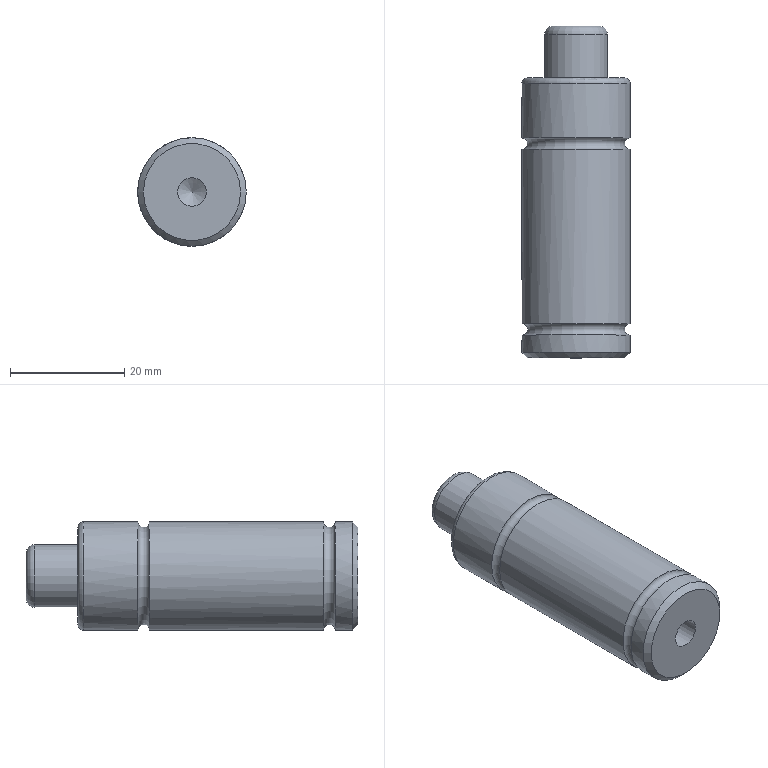Part | STEP file | 1_id822_x_t | 1 solid | 14 faces | box 19 x 58.09 x 19 mm | volume 14020 mm3 | cylinder 5 | torus 4 | plane 3 | cone 2 | commonest cylinder face diameters 19 x3 5 x1 11 x1
STEP:
#1=CARTESIAN_POINT('',(0.,0.,0.));
#2=DIRECTION('',(0.,0.,1.));
#3=DIRECTION('',(1.,0.,0.));
#4=AXIS2_PLACEMENT_3D('',#1,#2,#3);
#5=CARTESIAN_POINT('',(752.425,85.86,-84.184));
#6=VERTEX_POINT('',#5);
#7=CARTESIAN_POINT('',(747.425,85.86,-84.184));
#8=VERTEX_POINT('',#7);
#9=CARTESIAN_POINT('',(749.925,85.86,-84.184));
#10=DIRECTION('',(0.,-1.,0.));
#11=DIRECTION('',(-1.,0.,0.));
#12=AXIS2_PLACEMENT_3D('',#9,#10,#11);
#13=CIRCLE('',#12,2.5);
#14=CARTESIAN_POINT('',(749.925,86.563,-84.184));
#15=DIRECTION('',(0.,-1.,0.));
#16=DIRECTION('',(1.,0.,0.));
#17=AXIS2_PLACEMENT_3D('',#14,#15,#16);
#18=CONICAL_SURFACE('',#17,1.283,1.047);
#19=CARTESIAN_POINT('',(-3.142,0.7025));
#20=DIRECTION('',(1.,0.));
#21=VECTOR('',#20,1.);
#22=LINE('',#19,#21);
#23=(GEOMETRIC_REPRESENTATION_CONTEXT(2)PARAMETRIC_REPRESENTATION_CONTEXT()REPRESENTATION_CONTEXT('',''));
#24=DEFINITIONAL_REPRESENTATION('',(#22),#23);
#25=PCURVE('',#18,#24);
#26=CARTESIAN_POINT('',(749.925,80.86,-84.184));
#27=DIRECTION('',(0.,1.,0.));
#28=DIRECTION('',(1.,0.,0.));
#29=AXIS2_PLACEMENT_3D('',#26,#27,#28);
#30=CYLINDRICAL_SURFACE('',#29,2.5);
#31=CARTESIAN_POINT('',(9.425,5.));
#32=DIRECTION('',(-1.,0.));
#33=VECTOR('',#32,1.);
#34=LINE('',#31,#33);
#35=(GEOMETRIC_REPRESENTATION_CONTEXT(2)PARAMETRIC_REPRESENTATION_CONTEXT()REPRESENTATION_CONTEXT('',''));
#36=DEFINITIONAL_REPRESENTATION('',(#34),#35);
#37=PCURVE('',#30,#36);
#38=SURFACE_CURVE('',#13,(#25,#37),.PCURVE_S1.);
#39=EDGE_CURVE('',#6,#8,#38,.T.);
#40=ORIENTED_EDGE('',*,*,#39,.F.);
#41=CARTESIAN_POINT('',(749.925,87.304,-84.184));
#42=VERTEX_POINT('',#41);
#43=CARTESIAN_POINT('',(749.925,87.304,-84.184));
#44=CARTESIAN_POINT('',(752.425,85.86,-84.184));
#45=B_SPLINE_CURVE_WITH_KNOTS('',1,(#43,#44),.UNSPECIFIED.,.F.,.F.,(2,2),(-1.482,1.405),.PIECEWISE_BEZIER_KNOTS.);
#46=CARTESIAN_POINT('',(0.,0.));
#47=DIRECTION('',(0.,1.));
#48=VECTOR('',#47,1.);
#49=LINE('',#46,#48);
#50=(GEOMETRIC_REPRESENTATION_CONTEXT(2)PARAMETRIC_REPRESENTATION_CONTEXT()REPRESENTATION_CONTEXT('',''));
#51=DEFINITIONAL_REPRESENTATION('',(#49),#50);
#52=PCURVE('',#18,#51);
#53=CARTESIAN_POINT('',(6.283,0.));
#54=DIRECTION('',(0.,1.));
#55=VECTOR('',#54,1.);
#56=LINE('',#53,#55);
#57=(GEOMETRIC_REPRESENTATION_CONTEXT(2)PARAMETRIC_REPRESENTATION_CONTEXT()REPRESENTATION_CONTEXT('',''));
#58=DEFINITIONAL_REPRESENTATION('',(#56),#57);
#59=PCURVE('',#18,#58);
#60=SEAM_CURVE('',#45,(#52,#59),.PCURVE_S1.);
#61=EDGE_CURVE('',#42,#6,#60,.T.);
#62=ORIENTED_EDGE('',*,*,#61,.F.);
#63=ORIENTED_EDGE('',*,*,#61,.T.);
#64=CARTESIAN_POINT('',(749.925,85.86,-84.184));
#65=DIRECTION('',(0.,-1.,0.));
#66=DIRECTION('',(-1.,0.,0.));
#67=AXIS2_PLACEMENT_3D('',#64,#65,#66);
#68=CIRCLE('',#67,2.5);
#69=CARTESIAN_POINT('',(3.142,0.7025));
#70=DIRECTION('',(1.,0.));
#71=VECTOR('',#70,1.);
#72=LINE('',#69,#71);
#73=(GEOMETRIC_REPRESENTATION_CONTEXT(2)PARAMETRIC_REPRESENTATION_CONTEXT()REPRESENTATION_CONTEXT('',''));
#74=DEFINITIONAL_REPRESENTATION('',(#72),#73);
#75=PCURVE('',#18,#74);
#76=CARTESIAN_POINT('',(3.142,5.));
#77=DIRECTION('',(-1.,0.));
#78=VECTOR('',#77,1.);
#79=LINE('',#76,#78);
#80=(GEOMETRIC_REPRESENTATION_CONTEXT(2)PARAMETRIC_REPRESENTATION_CONTEXT()REPRESENTATION_CONTEXT('',''));
#81=DEFINITIONAL_REPRESENTATION('',(#79),#80);
#82=PCURVE('',#30,#81);
#83=SURFACE_CURVE('',#68,(#75,#82),.PCURVE_S1.);
#84=EDGE_CURVE('',#8,#6,#83,.T.);
#85=ORIENTED_EDGE('',*,*,#84,.F.);
#86=EDGE_LOOP('',(#40,#62,#63,#85));
#87=FACE_BOUND('',#86,.F.);
#88=ADVANCED_FACE('',(#87),#18,.F.);
#89=ORIENTED_EDGE('',*,*,#39,.T.);
#90=ORIENTED_EDGE('',*,*,#84,.T.);
#91=CARTESIAN_POINT('',(752.425,60.86,-84.184));
#92=VERTEX_POINT('',#91);
#93=CARTESIAN_POINT('',(752.425,60.86,-84.184));
#94=CARTESIAN_POINT('',(752.425,85.86,-84.184));
#95=B_SPLINE_CURVE_WITH_KNOTS('',1,(#93,#94),.UNSPECIFIED.,.F.,.F.,(2,2),(-20.,5.),.PIECEWISE_BEZIER_KNOTS.);
#96=CARTESIAN_POINT('',(0.,0.));
#97=DIRECTION('',(0.,1.));
#98=VECTOR('',#97,1.);
#99=LINE('',#96,#98);
#100=(GEOMETRIC_REPRESENTATION_CONTEXT(2)PARAMETRIC_REPRESENTATION_CONTEXT()REPRESENTATION_CONTEXT('',''));
#101=DEFINITIONAL_REPRESENTATION('',(#99),#100);
#102=PCURVE('',#30,#101);
#103=CARTESIAN_POINT('',(6.283,0.));
#104=DIRECTION('',(0.,1.));
#105=VECTOR('',#104,1.);
#106=LINE('',#103,#105);
#107=(GEOMETRIC_REPRESENTATION_CONTEXT(2)PARAMETRIC_REPRESENTATION_CONTEXT()REPRESENTATION_CONTEXT('',''));
#108=DEFINITIONAL_REPRESENTATION('',(#106),#107);
#109=PCURVE('',#30,#108);
#110=SEAM_CURVE('',#95,(#102,#109),.PCURVE_S1.);
#111=EDGE_CURVE('',#92,#6,#110,.T.);
#112=ORIENTED_EDGE('',*,*,#111,.F.);
#113=CARTESIAN_POINT('',(749.925,60.86,-84.184));
#114=DIRECTION('',(0.,1.,0.));
#115=DIRECTION('',(1.,0.,0.));
#116=AXIS2_PLACEMENT_3D('',#113,#114,#115);
#117=CIRCLE('',#116,2.5);
#118=CARTESIAN_POINT('',(0.,-20.));
#119=DIRECTION('',(1.,0.));
#120=VECTOR('',#119,1.);
#121=LINE('',#118,#120);
#122=(GEOMETRIC_REPRESENTATION_CONTEXT(2)PARAMETRIC_REPRESENTATION_CONTEXT()REPRESENTATION_CONTEXT('',''));
#123=DEFINITIONAL_REPRESENTATION('',(#121),#122);
#124=PCURVE('',#30,#123);
#125=CARTESIAN_POINT('',(749.925,60.86,-92.684));
#126=DIRECTION('',(0.,1.,0.));
#127=DIRECTION('',(1.,0.,0.));
#128=AXIS2_PLACEMENT_3D('',#125,#126,#127);
#129=PLANE('',#128);
#130=CARTESIAN_POINT('',(0.,-8.5));
#131=DIRECTION('',(1.,0.));
#132=AXIS2_PLACEMENT_2D('',#130,#131);
#133=CIRCLE('',#132,2.5);
#134=(GEOMETRIC_REPRESENTATION_CONTEXT(2)PARAMETRIC_REPRESENTATION_CONTEXT()REPRESENTATION_CONTEXT('',''));
#135=DEFINITIONAL_REPRESENTATION('',(#133),#134);
#136=PCURVE('',#129,#135);
#137=SURFACE_CURVE('',#117,(#124,#136),.PCURVE_S1.);
#138=EDGE_CURVE('',#92,#92,#137,.T.);
#139=ORIENTED_EDGE('',*,*,#138,.T.);
#140=ORIENTED_EDGE('',*,*,#111,.T.);
#141=EDGE_LOOP('',(#89,#90,#112,#139,#140));
#142=FACE_BOUND('',#141,.F.);
#143=ADVANCED_FACE('',(#142),#30,.F.);
#144=CARTESIAN_POINT('',(741.425,60.86,-84.184));
#145=VERTEX_POINT('',#144);
#146=CARTESIAN_POINT('',(749.925,60.86,-84.184));
#147=DIRECTION('',(0.,-1.,0.));
#148=DIRECTION('',(-1.,0.,0.));
#149=AXIS2_PLACEMENT_3D('',#146,#147,#148);
#150=CIRCLE('',#149,8.5);
#151=CARTESIAN_POINT('',(-8.5,-8.5));
#152=CARTESIAN_POINT('',(-8.5,6.222));
#153=CARTESIAN_POINT('',(4.25,-1.139));
#154=CARTESIAN_POINT('',(17.,-8.5));
#155=CARTESIAN_POINT('',(4.25,-15.861));
#156=CARTESIAN_POINT('',(-8.5,-23.222));
#157=CARTESIAN_POINT('',(-8.5,-8.5));
#158=(BOUNDED_CURVE()B_SPLINE_CURVE(2,(#151,#152,#153,#154,#155,#156,#157),.UNSPECIFIED.,.T.,.F.)B_SPLINE_CURVE_WITH_KNOTS((1,2,2,2,2,1),(-2.094,0.,2.094,4.189,6.283,8.378),.UNSPECIFIED.)CURVE()GEOMETRIC_REPRESENTATION_ITEM()RATIONAL_B_SPLINE_CURVE((1.,0.5,1.,0.5,1.,0.5,1.))REPRESENTATION_ITEM(''));
#159=(GEOMETRIC_REPRESENTATION_CONTEXT(2)PARAMETRIC_REPRESENTATION_CONTEXT()REPRESENTATION_CONTEXT('',''));
#160=DEFINITIONAL_REPRESENTATION('',(#158),#159);
#161=PCURVE('',#129,#160);
#162=CARTESIAN_POINT('',(749.925,61.36,-84.184));
#163=DIRECTION('',(0.,1.,0.));
#164=DIRECTION('',(-1.,0.,0.));
#165=AXIS2_PLACEMENT_3D('',#162,#163,#164);
#166=CONICAL_SURFACE('',#165,9.,0.7854);
#167=CARTESIAN_POINT('',(6.283,-0.5));
#168=DIRECTION('',(-1.,0.));
#169=VECTOR('',#168,1.);
#170=LINE('',#167,#169);
#171=(GEOMETRIC_REPRESENTATION_CONTEXT(2)PARAMETRIC_REPRESENTATION_CONTEXT()REPRESENTATION_CONTEXT('',''));
#172=DEFINITIONAL_REPRESENTATION('',(#170),#171);
#173=PCURVE('',#166,#172);
#174=SURFACE_CURVE('',#150,(#161,#173),.PCURVE_S1.);
#175=EDGE_CURVE('',#145,#145,#174,.T.);
#176=ORIENTED_EDGE('',*,*,#175,.T.);
#177=EDGE_LOOP('',(#176));
#178=FACE_BOUND('',#177,.T.);
#179=ORIENTED_EDGE('',*,*,#138,.T.);
#180=EDGE_LOOP('',(#179));
#181=FACE_BOUND('',#180,.T.);
#182=ADVANCED_FACE('',(#178,#181),#129,.F.);
#183=CARTESIAN_POINT('',(740.425,61.86,-84.184));
#184=VERTEX_POINT('',#183);
#185=CARTESIAN_POINT('',(759.425,61.86,-84.184));
#186=VERTEX_POINT('',#185);
#187=CARTESIAN_POINT('',(749.925,61.86,-84.184));
#188=DIRECTION('',(0.,-1.,0.));
#189=DIRECTION('',(-1.,0.,0.));
#190=AXIS2_PLACEMENT_3D('',#187,#188,#189);
#191=CIRCLE('',#190,9.5);
#192=CARTESIAN_POINT('',(6.283,0.5));
#193=DIRECTION('',(-1.,0.));
#194=VECTOR('',#193,1.);
#195=LINE('',#192,#194);
#196=(GEOMETRIC_REPRESENTATION_CONTEXT(2)PARAMETRIC_REPRESENTATION_CONTEXT()REPRESENTATION_CONTEXT('',''));
#197=DEFINITIONAL_REPRESENTATION('',(#195),#196);
#198=PCURVE('',#166,#197);
#199=CARTESIAN_POINT('',(749.925,104.86,-84.184));
#200=DIRECTION('',(0.,1.,0.));
#201=DIRECTION('',(1.,0.,0.));
#202=AXIS2_PLACEMENT_3D('',#199,#200,#201);
#203=CYLINDRICAL_SURFACE('',#202,9.5);
#204=CARTESIAN_POINT('',(3.142,-43.));
#205=DIRECTION('',(-1.,0.));
#206=VECTOR('',#205,1.);
#207=LINE('',#204,#206);
#208=(GEOMETRIC_REPRESENTATION_CONTEXT(2)PARAMETRIC_REPRESENTATION_CONTEXT()REPRESENTATION_CONTEXT('',''));
#209=DEFINITIONAL_REPRESENTATION('',(#207),#208);
#210=PCURVE('',#203,#209);
#211=SURFACE_CURVE('',#191,(#198,#210),.PCURVE_S1.);
#212=EDGE_CURVE('',#184,#186,#211,.T.);
#213=ORIENTED_EDGE('',*,*,#212,.T.);
#214=CARTESIAN_POINT('',(749.925,61.86,-84.184));
#215=DIRECTION('',(0.,-1.,0.));
#216=DIRECTION('',(-1.,0.,0.));
#217=AXIS2_PLACEMENT_3D('',#214,#215,#216);
#218=CIRCLE('',#217,9.5);
#219=CARTESIAN_POINT('',(6.283,0.5));
#220=DIRECTION('',(-1.,0.));
#221=VECTOR('',#220,1.);
#222=LINE('',#219,#221);
#223=(GEOMETRIC_REPRESENTATION_CONTEXT(2)PARAMETRIC_REPRESENTATION_CONTEXT()REPRESENTATION_CONTEXT('',''));
#224=DEFINITIONAL_REPRESENTATION('',(#222),#223);
#225=PCURVE('',#166,#224);
#226=CARTESIAN_POINT('',(9.425,-43.));
#227=DIRECTION('',(-1.,0.));
#228=VECTOR('',#227,1.);
#229=LINE('',#226,#228);
#230=(GEOMETRIC_REPRESENTATION_CONTEXT(2)PARAMETRIC_REPRESENTATION_CONTEXT()REPRESENTATION_CONTEXT('',''));
#231=DEFINITIONAL_REPRESENTATION('',(#229),#230);
#232=PCURVE('',#203,#231);
#233=SURFACE_CURVE('',#218,(#225,#232),.PCURVE_S1.);
#234=EDGE_CURVE('',#186,#184,#233,.T.);
#235=ORIENTED_EDGE('',*,*,#234,.T.);
#236=CARTESIAN_POINT('',(741.425,60.86,-84.184));
#237=CARTESIAN_POINT('',(740.425,61.86,-84.184));
#238=B_SPLINE_CURVE_WITH_KNOTS('',1,(#236,#237),.UNSPECIFIED.,.F.,.F.,(2,2),(-0.7071,0.7071),.PIECEWISE_BEZIER_KNOTS.);
#239=CARTESIAN_POINT('',(0.,0.));
#240=DIRECTION('',(0.,1.));
#241=VECTOR('',#240,1.);
#242=LINE('',#239,#241);
#243=(GEOMETRIC_REPRESENTATION_CONTEXT(2)PARAMETRIC_REPRESENTATION_CONTEXT()REPRESENTATION_CONTEXT('',''));
#244=DEFINITIONAL_REPRESENTATION('',(#242),#243);
#245=PCURVE('',#166,#244);
#246=CARTESIAN_POINT('',(6.283,0.));
#247=DIRECTION('',(0.,1.));
#248=VECTOR('',#247,1.);
#249=LINE('',#246,#248);
#250=(GEOMETRIC_REPRESENTATION_CONTEXT(2)PARAMETRIC_REPRESENTATION_CONTEXT()REPRESENTATION_CONTEXT('',''));
#251=DEFINITIONAL_REPRESENTATION('',(#249),#250);
#252=PCURVE('',#166,#251);
#253=SEAM_CURVE('',#238,(#245,#252),.PCURVE_S1.);
#254=EDGE_CURVE('',#145,#184,#253,.T.);
#255=ORIENTED_EDGE('',*,*,#254,.F.);
#256=ORIENTED_EDGE('',*,*,#175,.F.);
#257=ORIENTED_EDGE('',*,*,#254,.T.);
#258=EDGE_LOOP('',(#213,#235,#255,#256,#257));
#259=FACE_BOUND('',#258,.T.);
#260=ADVANCED_FACE('',(#259),#166,.T.);
#261=CARTESIAN_POINT('',(759.425,64.86,-84.184));
#262=VERTEX_POINT('',#261);
#263=CARTESIAN_POINT('',(749.925,64.86,-84.184));
#264=DIRECTION('',(0.,1.,0.));
#265=DIRECTION('',(1.,0.,0.));
#266=AXIS2_PLACEMENT_3D('',#263,#264,#265);
#267=CIRCLE('',#266,9.5);
#268=CARTESIAN_POINT('',(0.,-40.));
#269=DIRECTION('',(1.,0.));
#270=VECTOR('',#269,1.);
#271=LINE('',#268,#270);
#272=(GEOMETRIC_REPRESENTATION_CONTEXT(2)PARAMETRIC_REPRESENTATION_CONTEXT()REPRESENTATION_CONTEXT('',''));
#273=DEFINITIONAL_REPRESENTATION('',(#271),#272);
#274=PCURVE('',#203,#273);
#275=CARTESIAN_POINT('',(749.925,65.86,-84.184));
#276=DIRECTION('',(0.,-1.,0.));
#277=DIRECTION('',(1.,0.,0.));
#278=AXIS2_PLACEMENT_3D('',#275,#276,#277);
#279=TOROIDAL_SURFACE('',#278,9.5,1.);
#280=CARTESIAN_POINT('',(6.283,1.571));
#281=DIRECTION('',(-1.,0.));
#282=VECTOR('',#281,1.);
#283=LINE('',#280,#282);
#284=(GEOMETRIC_REPRESENTATION_CONTEXT(2)PARAMETRIC_REPRESENTATION_CONTEXT()REPRESENTATION_CONTEXT('',''));
#285=DEFINITIONAL_REPRESENTATION('',(#283),#284);
#286=PCURVE('',#279,#285);
#287=SURFACE_CURVE('',#267,(#274,#286),.PCURVE_S1.);
#288=EDGE_CURVE('',#262,#262,#287,.T.);
#289=ORIENTED_EDGE('',*,*,#288,.F.);
#290=CARTESIAN_POINT('',(759.425,61.86,-84.184));
#291=CARTESIAN_POINT('',(759.425,64.86,-84.184));
#292=B_SPLINE_CURVE_WITH_KNOTS('',1,(#290,#291),.UNSPECIFIED.,.F.,.F.,(2,2),(-43.,-40.),.PIECEWISE_BEZIER_KNOTS.);
#293=CARTESIAN_POINT('',(0.,0.));
#294=DIRECTION('',(0.,1.));
#295=VECTOR('',#294,1.);
#296=LINE('',#293,#295);
#297=(GEOMETRIC_REPRESENTATION_CONTEXT(2)PARAMETRIC_REPRESENTATION_CONTEXT()REPRESENTATION_CONTEXT('',''));
#298=DEFINITIONAL_REPRESENTATION('',(#296),#297);
#299=PCURVE('',#203,#298);
#300=CARTESIAN_POINT('',(6.283,0.));
#301=DIRECTION('',(0.,1.));
#302=VECTOR('',#301,1.);
#303=LINE('',#300,#302);
#304=(GEOMETRIC_REPRESENTATION_CONTEXT(2)PARAMETRIC_REPRESENTATION_CONTEXT()REPRESENTATION_CONTEXT('',''));
#305=DEFINITIONAL_REPRESENTATION('',(#303),#304);
#306=PCURVE('',#203,#305);
#307=SEAM_CURVE('',#292,(#299,#306),.PCURVE_S1.);
#308=EDGE_CURVE('',#186,#262,#307,.T.);
#309=ORIENTED_EDGE('',*,*,#308,.F.);
#310=ORIENTED_EDGE('',*,*,#212,.F.);
#311=ORIENTED_EDGE('',*,*,#234,.F.);
#312=ORIENTED_EDGE('',*,*,#308,.T.);
#313=EDGE_LOOP('',(#289,#309,#310,#311,#312));
#314=FACE_BOUND('',#313,.T.);
#315=ADVANCED_FACE('',(#314),#203,.T.);
#316=CARTESIAN_POINT('',(759.425,66.86,-84.184));
#317=VERTEX_POINT('',#316);
#318=CARTESIAN_POINT('',(749.925,66.86,-84.184));
#319=DIRECTION('',(0.,-1.,0.));
#320=DIRECTION('',(1.,0.,0.));
#321=AXIS2_PLACEMENT_3D('',#318,#319,#320);
#322=CIRCLE('',#321,9.5);
#323=CARTESIAN_POINT('',(0.,4.712));
#324=DIRECTION('',(1.,0.));
#325=VECTOR('',#324,1.);
#326=LINE('',#323,#325);
#327=(GEOMETRIC_REPRESENTATION_CONTEXT(2)PARAMETRIC_REPRESENTATION_CONTEXT()REPRESENTATION_CONTEXT('',''));
#328=DEFINITIONAL_REPRESENTATION('',(#326),#327);
#329=PCURVE('',#279,#328);
#330=CARTESIAN_POINT('',(749.925,104.86,-84.184));
#331=DIRECTION('',(0.,1.,0.));
#332=DIRECTION('',(1.,0.,0.));
#333=AXIS2_PLACEMENT_3D('',#330,#331,#332);
#334=CYLINDRICAL_SURFACE('',#333,9.5);
#335=CARTESIAN_POINT('',(6.283,-38.));
#336=DIRECTION('',(-1.,0.));
#337=VECTOR('',#336,1.);
#338=LINE('',#335,#337);
#339=(GEOMETRIC_REPRESENTATION_CONTEXT(2)PARAMETRIC_REPRESENTATION_CONTEXT()REPRESENTATION_CONTEXT('',''));
#340=DEFINITIONAL_REPRESENTATION('',(#338),#339);
#341=PCURVE('',#334,#340);
#342=SURFACE_CURVE('',#322,(#329,#341),.PCURVE_S1.);
#343=EDGE_CURVE('',#317,#317,#342,.T.);
#344=ORIENTED_EDGE('',*,*,#343,.F.);
#345=CARTESIAN_POINT('',(759.425,64.86,-84.184));
#346=CARTESIAN_POINT('',(759.032,64.86,-84.184));
#347=CARTESIAN_POINT('',(758.64,65.036,-84.184));
#348=CARTESIAN_POINT('',(758.339,65.389,-84.184));
#349=CARTESIAN_POINT('',(758.223,65.86,-84.184));
#350=CARTESIAN_POINT('',(758.339,66.332,-84.184));
#351=CARTESIAN_POINT('',(758.64,66.684,-84.184));
#352=CARTESIAN_POINT('',(759.032,66.86,-84.184));
#353=CARTESIAN_POINT('',(759.425,66.86,-84.184));
#354=B_SPLINE_CURVE_WITH_KNOTS('',8,(#345,#346,#347,#348,#349,#350,#351,#352,#353),.UNSPECIFIED.,.F.,.F.,(9,9),(1.571,4.712),.PIECEWISE_BEZIER_KNOTS.);
#355=CARTESIAN_POINT('',(0.,0.));
#356=DIRECTION('',(0.,1.));
#357=VECTOR('',#356,1.);
#358=LINE('',#355,#357);
#359=(GEOMETRIC_REPRESENTATION_CONTEXT(2)PARAMETRIC_REPRESENTATION_CONTEXT()REPRESENTATION_CONTEXT('',''));
#360=DEFINITIONAL_REPRESENTATION('',(#358),#359);
#361=PCURVE('',#279,#360);
#362=CARTESIAN_POINT('',(6.283,0.));
#363=DIRECTION('',(0.,1.));
#364=VECTOR('',#363,1.);
#365=LINE('',#362,#364);
#366=(GEOMETRIC_REPRESENTATION_CONTEXT(2)PARAMETRIC_REPRESENTATION_CONTEXT()REPRESENTATION_CONTEXT('',''));
#367=DEFINITIONAL_REPRESENTATION('',(#365),#366);
#368=PCURVE('',#279,#367);
#369=SEAM_CURVE('',#354,(#361,#368),.PCURVE_S1.);
#370=EDGE_CURVE('',#262,#317,#369,.T.);
#371=ORIENTED_EDGE('',*,*,#370,.F.);
#372=ORIENTED_EDGE('',*,*,#288,.F.);
#373=ORIENTED_EDGE('',*,*,#370,.T.);
#374=EDGE_LOOP('',(#344,#371,#372,#373));
#375=FACE_BOUND('',#374,.F.);
#376=ADVANCED_FACE('',(#375),#279,.F.);
#377=CARTESIAN_POINT('',(759.425,97.36,-84.184));
#378=VERTEX_POINT('',#377);
#379=CARTESIAN_POINT('',(740.425,97.36,-84.184));
#380=VERTEX_POINT('',#379);
#381=CARTESIAN_POINT('',(749.925,97.36,-84.184));
#382=DIRECTION('',(0.,1.,0.));
#383=DIRECTION('',(-1.,0.,0.));
#384=AXIS2_PLACEMENT_3D('',#381,#382,#383);
#385=CIRCLE('',#384,9.5);
#386=CARTESIAN_POINT('',(-3.142,-7.5));
#387=DIRECTION('',(1.,0.));
#388=VECTOR('',#387,1.);
#389=LINE('',#386,#388);
#390=(GEOMETRIC_REPRESENTATION_CONTEXT(2)PARAMETRIC_REPRESENTATION_CONTEXT()REPRESENTATION_CONTEXT('',''));
#391=DEFINITIONAL_REPRESENTATION('',(#389),#390);
#392=PCURVE('',#334,#391);
#393=CARTESIAN_POINT('',(749.925,98.36,-84.184));
#394=DIRECTION('',(0.,-1.,0.));
#395=DIRECTION('',(1.,0.,0.));
#396=AXIS2_PLACEMENT_3D('',#393,#394,#395);
#397=TOROIDAL_SURFACE('',#396,9.5,1.);
#398=CARTESIAN_POINT('',(9.425,1.571));
#399=DIRECTION('',(-1.,0.));
#400=VECTOR('',#399,1.);
#401=LINE('',#398,#400);
#402=(GEOMETRIC_REPRESENTATION_CONTEXT(2)PARAMETRIC_REPRESENTATION_CONTEXT()REPRESENTATION_CONTEXT('',''));
#403=DEFINITIONAL_REPRESENTATION('',(#401),#402);
#404=PCURVE('',#397,#403);
#405=SURFACE_CURVE('',#385,(#392,#404),.PCURVE_S1.);
#406=EDGE_CURVE('',#378,#380,#405,.T.);
#407=ORIENTED_EDGE('',*,*,#406,.F.);
#408=CARTESIAN_POINT('',(759.425,66.86,-84.184));
#409=CARTESIAN_POINT('',(759.425,97.36,-84.184));
#410=B_SPLINE_CURVE_WITH_KNOTS('',1,(#408,#409),.UNSPECIFIED.,.F.,.F.,(2,2),(-38.,-7.5),.PIECEWISE_BEZIER_KNOTS.);
#411=CARTESIAN_POINT('',(0.,0.));
#412=DIRECTION('',(0.,1.));
#413=VECTOR('',#412,1.);
#414=LINE('',#411,#413);
#415=(GEOMETRIC_REPRESENTATION_CONTEXT(2)PARAMETRIC_REPRESENTATION_CONTEXT()REPRESENTATION_CONTEXT('',''));
#416=DEFINITIONAL_REPRESENTATION('',(#414),#415);
#417=PCURVE('',#334,#416);
#418=CARTESIAN_POINT('',(6.283,0.));
#419=DIRECTION('',(0.,1.));
#420=VECTOR('',#419,1.);
#421=LINE('',#418,#420);
#422=(GEOMETRIC_REPRESENTATION_CONTEXT(2)PARAMETRIC_REPRESENTATION_CONTEXT()REPRESENTATION_CONTEXT('',''));
#423=DEFINITIONAL_REPRESENTATION('',(#421),#422);
#424=PCURVE('',#334,#423);
#425=SEAM_CURVE('',#410,(#417,#424),.PCURVE_S1.);
#426=EDGE_CURVE('',#317,#378,#425,.T.);
#427=ORIENTED_EDGE('',*,*,#426,.F.);
#428=ORIENTED_EDGE('',*,*,#343,.F.);
#429=ORIENTED_EDGE('',*,*,#426,.T.);
#430=CARTESIAN_POINT('',(749.925,97.36,-84.184));
#431=DIRECTION('',(0.,1.,0.));
#432=DIRECTION('',(-1.,0.,0.));
#433=AXIS2_PLACEMENT_3D('',#430,#431,#432);
#434=CIRCLE('',#433,9.5);
#435=CARTESIAN_POINT('',(3.142,-7.5));
#436=DIRECTION('',(1.,0.));
#437=VECTOR('',#436,1.);
#438=LINE('',#435,#437);
#439=(GEOMETRIC_REPRESENTATION_CONTEXT(2)PARAMETRIC_REPRESENTATION_CONTEXT()REPRESENTATION_CONTEXT('',''));
#440=DEFINITIONAL_REPRESENTATION('',(#438),#439);
#441=PCURVE('',#334,#440);
#442=CARTESIAN_POINT('',(9.425,1.571));
#443=DIRECTION('',(-1.,0.));
#444=VECTOR('',#443,1.);
#445=LINE('',#442,#444);
#446=(GEOMETRIC_REPRESENTATION_CONTEXT(2)PARAMETRIC_REPRESENTATION_CONTEXT()REPRESENTATION_CONTEXT('',''));
#447=DEFINITIONAL_REPRESENTATION('',(#445),#446);
#448=PCURVE('',#397,#447);
#449=SURFACE_CURVE('',#434,(#441,#448),.PCURVE_S1.);
#450=EDGE_CURVE('',#380,#378,#449,.T.);
#451=ORIENTED_EDGE('',*,*,#450,.F.);
#452=EDGE_LOOP('',(#407,#427,#428,#429,#451));
#453=FACE_BOUND('',#452,.T.);
#454=ADVANCED_FACE('',(#453),#334,.T.);
#455=CARTESIAN_POINT('',(740.425,99.36,-84.184));
#456=VERTEX_POINT('',#455);
#457=CARTESIAN_POINT('',(759.425,99.36,-84.184));
#458=VERTEX_POINT('',#457);
#459=CARTESIAN_POINT('',(749.925,99.36,-84.184));
#460=DIRECTION('',(0.,-1.,0.));
#461=DIRECTION('',(-1.,0.,0.));
#462=AXIS2_PLACEMENT_3D('',#459,#460,#461);
#463=CIRCLE('',#462,9.5);
#464=CARTESIAN_POINT('',(3.142,4.712));
#465=DIRECTION('',(1.,0.));
#466=VECTOR('',#465,1.);
#467=LINE('',#464,#466);
#468=(GEOMETRIC_REPRESENTATION_CONTEXT(2)PARAMETRIC_REPRESENTATION_CONTEXT()REPRESENTATION_CONTEXT('',''));
#469=DEFINITIONAL_REPRESENTATION('',(#467),#468);
#470=PCURVE('',#397,#469);
#471=CARTESIAN_POINT('',(749.925,109.86,-84.184));
#472=DIRECTION('',(0.,1.,0.));
#473=DIRECTION('',(1.,0.,0.));
#474=AXIS2_PLACEMENT_3D('',#471,#472,#473);
#475=CYLINDRICAL_SURFACE('',#474,9.5);
#476=CARTESIAN_POINT('',(3.142,-10.5));
#477=DIRECTION('',(-1.,0.));
#478=VECTOR('',#477,1.);
#479=LINE('',#476,#478);
#480=(GEOMETRIC_REPRESENTATION_CONTEXT(2)PARAMETRIC_REPRESENTATION_CONTEXT()REPRESENTATION_CONTEXT('',''));
#481=DEFINITIONAL_REPRESENTATION('',(#479),#480);
#482=PCURVE('',#475,#481);
#483=SURFACE_CURVE('',#463,(#470,#482),.PCURVE_S1.);
#484=EDGE_CURVE('',#456,#458,#483,.T.);
#485=ORIENTED_EDGE('',*,*,#484,.F.);
#486=CARTESIAN_POINT('',(740.425,97.36,-84.184));
#487=CARTESIAN_POINT('',(740.818,97.36,-84.184));
#488=CARTESIAN_POINT('',(741.21,97.536,-84.184));
#489=CARTESIAN_POINT('',(741.511,97.889,-84.184));
#490=CARTESIAN_POINT('',(741.627,98.36,-84.184));
#491=CARTESIAN_POINT('',(741.511,98.832,-84.184));
#492=CARTESIAN_POINT('',(741.21,99.184,-84.184));
#493=CARTESIAN_POINT('',(740.818,99.36,-84.184));
#494=CARTESIAN_POINT('',(740.425,99.36,-84.184));
#495=B_SPLINE_CURVE_WITH_KNOTS('',8,(#486,#487,#488,#489,#490,#491,#492,#493,#494),.UNSPECIFIED.,.F.,.F.,(9,9),(1.571,4.712),.PIECEWISE_BEZIER_KNOTS.);
#496=CARTESIAN_POINT('',(3.142,0.));
#497=DIRECTION('',(0.,1.));
#498=VECTOR('',#497,1.);
#499=LINE('',#496,#498);
#500=(GEOMETRIC_REPRESENTATION_CONTEXT(2)PARAMETRIC_REPRESENTATION_CONTEXT()REPRESENTATION_CONTEXT('',''));
#501=DEFINITIONAL_REPRESENTATION('',(#499),#500);
#502=PCURVE('',#397,#501);
#503=CARTESIAN_POINT('',(9.425,0.));
#504=DIRECTION('',(0.,1.));
#505=VECTOR('',#504,1.);
#506=LINE('',#503,#505);
#507=(GEOMETRIC_REPRESENTATION_CONTEXT(2)PARAMETRIC_REPRESENTATION_CONTEXT()REPRESENTATION_CONTEXT('',''));
#508=DEFINITIONAL_REPRESENTATION('',(#506),#507);
#509=PCURVE('',#397,#508);
#510=SEAM_CURVE('',#495,(#502,#509),.PCURVE_S1.);
#511=EDGE_CURVE('',#380,#456,#510,.T.);
#512=ORIENTED_EDGE('',*,*,#511,.F.);
#513=ORIENTED_EDGE('',*,*,#406,.F.);
#514=ORIENTED_EDGE('',*,*,#450,.F.);
#515=ORIENTED_EDGE('',*,*,#511,.T.);
#516=CARTESIAN_POINT('',(749.925,99.36,-84.184));
#517=DIRECTION('',(0.,-1.,0.));
#518=DIRECTION('',(-1.,0.,0.));
#519=AXIS2_PLACEMENT_3D('',#516,#517,#518);
#520=CIRCLE('',#519,9.5);
#521=CARTESIAN_POINT('',(3.142,4.712));
#522=DIRECTION('',(1.,0.));
#523=VECTOR('',#522,1.);
#524=LINE('',#521,#523);
#525=(GEOMETRIC_REPRESENTATION_CONTEXT(2)PARAMETRIC_REPRESENTATION_CONTEXT()REPRESENTATION_CONTEXT('',''));
#526=DEFINITIONAL_REPRESENTATION('',(#524),#525);
#527=PCURVE('',#397,#526);
#528=CARTESIAN_POINT('',(9.425,-10.5));
#529=DIRECTION('',(-1.,0.));
#530=VECTOR('',#529,1.);
#531=LINE('',#528,#530);
#532=(GEOMETRIC_REPRESENTATION_CONTEXT(2)PARAMETRIC_REPRESENTATION_CONTEXT()REPRESENTATION_CONTEXT('',''));
#533=DEFINITIONAL_REPRESENTATION('',(#531),#532);
#534=PCURVE('',#475,#533);
#535=SURFACE_CURVE('',#520,(#527,#534),.PCURVE_S1.);
#536=EDGE_CURVE('',#458,#456,#535,.T.);
#537=ORIENTED_EDGE('',*,*,#536,.F.);
#538=EDGE_LOOP('',(#485,#512,#513,#514,#515,#537));
#539=FACE_BOUND('',#538,.F.);
#540=ADVANCED_FACE('',(#539),#397,.F.);
#541=CARTESIAN_POINT('',(759.425,108.86,-84.184));
#542=VERTEX_POINT('',#541);
#543=CARTESIAN_POINT('',(749.925,108.86,-84.184));
#544=DIRECTION('',(0.,1.,0.));
#545=DIRECTION('',(1.,0.,0.));
#546=AXIS2_PLACEMENT_3D('',#543,#544,#545);
#547=CIRCLE('',#546,9.5);
#548=CARTESIAN_POINT('',(0.,-1.));
#549=DIRECTION('',(1.,0.));
#550=VECTOR('',#549,1.);
#551=LINE('',#548,#550);
#552=(GEOMETRIC_REPRESENTATION_CONTEXT(2)PARAMETRIC_REPRESENTATION_CONTEXT()REPRESENTATION_CONTEXT('',''));
#553=DEFINITIONAL_REPRESENTATION('',(#551),#552);
#554=PCURVE('',#475,#553);
#555=CARTESIAN_POINT('',(749.925,108.86,-84.184));
#556=DIRECTION('',(0.,-1.,0.));
#557=DIRECTION('',(1.,0.,0.));
#558=AXIS2_PLACEMENT_3D('',#555,#556,#557);
#559=TOROIDAL_SURFACE('',#558,8.5,1.);
#560=CARTESIAN_POINT('',(6.283,6.283));
#561=DIRECTION('',(-1.,0.));
#562=VECTOR('',#561,1.);
#563=LINE('',#560,#562);
#564=(GEOMETRIC_REPRESENTATION_CONTEXT(2)PARAMETRIC_REPRESENTATION_CONTEXT()REPRESENTATION_CONTEXT('',''));
#565=DEFINITIONAL_REPRESENTATION('',(#563),#564);
#566=PCURVE('',#559,#565);
#567=SURFACE_CURVE('',#547,(#554,#566),.PCURVE_S1.);
#568=EDGE_CURVE('',#542,#542,#567,.T.);
#569=ORIENTED_EDGE('',*,*,#568,.F.);
#570=CARTESIAN_POINT('',(759.425,99.36,-84.184));
#571=CARTESIAN_POINT('',(759.425,108.86,-84.184));
#572=B_SPLINE_CURVE_WITH_KNOTS('',1,(#570,#571),.UNSPECIFIED.,.F.,.F.,(2,2),(-10.5,-1.),.PIECEWISE_BEZIER_KNOTS.);
#573=CARTESIAN_POINT('',(0.,0.));
#574=DIRECTION('',(0.,1.));
#575=VECTOR('',#574,1.);
#576=LINE('',#573,#575);
#577=(GEOMETRIC_REPRESENTATION_CONTEXT(2)PARAMETRIC_REPRESENTATION_CONTEXT()REPRESENTATION_CONTEXT('',''));
#578=DEFINITIONAL_REPRESENTATION('',(#576),#577);
#579=PCURVE('',#475,#578);
#580=CARTESIAN_POINT('',(6.283,0.));
#581=DIRECTION('',(0.,1.));
#582=VECTOR('',#581,1.);
#583=LINE('',#580,#582);
#584=(GEOMETRIC_REPRESENTATION_CONTEXT(2)PARAMETRIC_REPRESENTATION_CONTEXT()REPRESENTATION_CONTEXT('',''));
#585=DEFINITIONAL_REPRESENTATION('',(#583),#584);
#586=PCURVE('',#475,#585);
#587=SEAM_CURVE('',#572,(#579,#586),.PCURVE_S1.);
#588=EDGE_CURVE('',#458,#542,#587,.T.);
#589=ORIENTED_EDGE('',*,*,#588,.F.);
#590=ORIENTED_EDGE('',*,*,#484,.F.);
#591=ORIENTED_EDGE('',*,*,#536,.F.);
#592=ORIENTED_EDGE('',*,*,#588,.T.);
#593=EDGE_LOOP('',(#569,#589,#590,#591,#592));
#594=FACE_BOUND('',#593,.T.);
#595=ADVANCED_FACE('',(#594),#475,.T.);
#596=ORIENTED_EDGE('',*,*,#568,.T.);
#597=CARTESIAN_POINT('',(758.425,109.86,-84.184));
#598=VERTEX_POINT('',#597);
#599=CARTESIAN_POINT('',(758.425,109.86,-84.184));
#600=CARTESIAN_POINT('',(758.692,109.86,-84.184));
#601=CARTESIAN_POINT('',(758.953,109.775,-84.184));
#602=CARTESIAN_POINT('',(759.177,109.612,-84.184));
#603=CARTESIAN_POINT('',(759.34,109.388,-84.184));
#604=CARTESIAN_POINT('',(759.425,109.128,-84.184));
#605=CARTESIAN_POINT('',(759.425,108.86,-84.184));
#606=(BOUNDED_CURVE()B_SPLINE_CURVE(6,(#599,#600,#601,#602,#603,#604,#605),.UNSPECIFIED.,.F.,.F.)B_SPLINE_CURVE_WITH_KNOTS((7,7),(-1.571,0.),.PIECEWISE_BEZIER_KNOTS.)CURVE()GEOMETRIC_REPRESENTATION_ITEM()RATIONAL_B_SPLINE_CURVE((1.031,1.01,0.9979,0.994,0.9979,1.01,1.031))REPRESENTATION_ITEM(''));
#607=CARTESIAN_POINT('',(0.,6.283));
#608=DIRECTION('',(0.,1.));
#609=VECTOR('',#608,1.);
#610=LINE('',#607,#609);
#611=(GEOMETRIC_REPRESENTATION_CONTEXT(2)PARAMETRIC_REPRESENTATION_CONTEXT()REPRESENTATION_CONTEXT('',''));
#612=DEFINITIONAL_REPRESENTATION('',(#610),#611);
#613=PCURVE('',#559,#612);
#614=CARTESIAN_POINT('',(6.283,6.283));
#615=DIRECTION('',(0.,1.));
#616=VECTOR('',#615,1.);
#617=LINE('',#614,#616);
#618=(GEOMETRIC_REPRESENTATION_CONTEXT(2)PARAMETRIC_REPRESENTATION_CONTEXT()REPRESENTATION_CONTEXT('',''));
#619=DEFINITIONAL_REPRESENTATION('',(#617),#618);
#620=PCURVE('',#559,#619);
#621=SEAM_CURVE('',#606,(#613,#620),.PCURVE_S1.);
#622=EDGE_CURVE('',#598,#542,#621,.T.);
#623=ORIENTED_EDGE('',*,*,#622,.F.);
#624=CARTESIAN_POINT('',(741.425,109.86,-84.184));
#625=VERTEX_POINT('',#624);
#626=CARTESIAN_POINT('',(749.925,109.86,-84.184));
#627=DIRECTION('',(0.,1.,0.));
#628=DIRECTION('',(-1.,0.,0.));
#629=AXIS2_PLACEMENT_3D('',#626,#627,#628);
#630=CIRCLE('',#629,8.5);
#631=CARTESIAN_POINT('',(3.142,4.712));
#632=DIRECTION('',(-1.,0.));
#633=VECTOR('',#632,1.);
#634=LINE('',#631,#633);
#635=(GEOMETRIC_REPRESENTATION_CONTEXT(2)PARAMETRIC_REPRESENTATION_CONTEXT()REPRESENTATION_CONTEXT('',''));
#636=DEFINITIONAL_REPRESENTATION('',(#634),#635);
#637=PCURVE('',#559,#636);
#638=CARTESIAN_POINT('',(749.925,109.86,-89.684));
#639=DIRECTION('',(0.,-1.,0.));
#640=DIRECTION('',(-1.,0.,0.));
#641=AXIS2_PLACEMENT_3D('',#638,#639,#640);
#642=PLANE('',#641);
#643=CARTESIAN_POINT('',(8.5,-5.5));
#644=CARTESIAN_POINT('',(8.5,-20.222));
#645=CARTESIAN_POINT('',(-4.25,-12.861));
#646=CARTESIAN_POINT('',(-17.,-5.5));
#647=CARTESIAN_POINT('',(-4.25,1.861));
#648=CARTESIAN_POINT('',(8.5,9.222));
#649=CARTESIAN_POINT('',(8.5,-5.5));
#650=(BOUNDED_CURVE()B_SPLINE_CURVE(2,(#643,#644,#645,#646,#647,#648,#649),.UNSPECIFIED.,.T.,.F.)B_SPLINE_CURVE_WITH_KNOTS((1,2,2,2,2,1),(-2.094,0.,2.094,4.189,6.283,8.378),.UNSPECIFIED.)CURVE()GEOMETRIC_REPRESENTATION_ITEM()RATIONAL_B_SPLINE_CURVE((1.,0.5,1.,0.5,1.,0.5,1.))REPRESENTATION_ITEM(''));
#651=(GEOMETRIC_REPRESENTATION_CONTEXT(2)PARAMETRIC_REPRESENTATION_CONTEXT()REPRESENTATION_CONTEXT('',''));
#652=DEFINITIONAL_REPRESENTATION('',(#650),#651);
#653=PCURVE('',#642,#652);
#654=SURFACE_CURVE('',#630,(#637,#653),.PCURVE_S1.);
#655=EDGE_CURVE('',#625,#598,#654,.T.);
#656=ORIENTED_EDGE('',*,*,#655,.F.);
#657=CARTESIAN_POINT('',(749.925,109.86,-84.184));
#658=DIRECTION('',(0.,1.,0.));
#659=DIRECTION('',(-1.,0.,0.));
#660=AXIS2_PLACEMENT_3D('',#657,#658,#659);
#661=CIRCLE('',#660,8.5);
#662=CARTESIAN_POINT('',(9.425,4.712));
#663=DIRECTION('',(-1.,0.));
#664=VECTOR('',#663,1.);
#665=LINE('',#662,#664);
#666=(GEOMETRIC_REPRESENTATION_CONTEXT(2)PARAMETRIC_REPRESENTATION_CONTEXT()REPRESENTATION_CONTEXT('',''));
#667=DEFINITIONAL_REPRESENTATION('',(#665),#666);
#668=PCURVE('',#559,#667);
#669=CARTESIAN_POINT('',(8.5,-5.5));
#670=CARTESIAN_POINT('',(8.5,-20.222));
#671=CARTESIAN_POINT('',(-4.25,-12.861));
#672=CARTESIAN_POINT('',(-17.,-5.5));
#673=CARTESIAN_POINT('',(-4.25,1.861));
#674=CARTESIAN_POINT('',(8.5,9.222));
#675=CARTESIAN_POINT('',(8.5,-5.5));
#676=(BOUNDED_CURVE()B_SPLINE_CURVE(2,(#669,#670,#671,#672,#673,#674,#675),.UNSPECIFIED.,.T.,.F.)B_SPLINE_CURVE_WITH_KNOTS((1,2,2,2,2,1),(-2.094,0.,2.094,4.189,6.283,8.378),.UNSPECIFIED.)CURVE()GEOMETRIC_REPRESENTATION_ITEM()RATIONAL_B_SPLINE_CURVE((1.,0.5,1.,0.5,1.,0.5,1.))REPRESENTATION_ITEM(''));
#677=(GEOMETRIC_REPRESENTATION_CONTEXT(2)PARAMETRIC_REPRESENTATION_CONTEXT()REPRESENTATION_CONTEXT('',''));
#678=DEFINITIONAL_REPRESENTATION('',(#676),#677);
#679=PCURVE('',#642,#678);
#680=SURFACE_CURVE('',#661,(#668,#679),.PCURVE_S1.);
#681=EDGE_CURVE('',#598,#625,#680,.T.);
#682=ORIENTED_EDGE('',*,*,#681,.F.);
#683=ORIENTED_EDGE('',*,*,#622,.T.);
#684=EDGE_LOOP('',(#596,#623,#656,#682,#683));
#685=FACE_BOUND('',#684,.T.);
#686=ADVANCED_FACE('',(#685),#559,.T.);
#687=ORIENTED_EDGE('',*,*,#655,.T.);
#688=ORIENTED_EDGE('',*,*,#681,.T.);
#689=EDGE_LOOP('',(#687,#688));
#690=FACE_BOUND('',#689,.T.);
#691=CARTESIAN_POINT('',(744.425,109.86,-84.184));
#692=VERTEX_POINT('',#691);
#693=CARTESIAN_POINT('',(755.425,109.86,-84.184));
#694=VERTEX_POINT('',#693);
#695=CARTESIAN_POINT('',(749.925,109.86,-84.184));
#696=DIRECTION('',(0.,-1.,0.));
#697=DIRECTION('',(-1.,0.,0.));
#698=AXIS2_PLACEMENT_3D('',#695,#696,#697);
#699=CIRCLE('',#698,5.5);
#700=CARTESIAN_POINT('',(0.,-5.5));
#701=DIRECTION('',(1.,0.));
#702=AXIS2_PLACEMENT_2D('',#700,#701);
#703=CIRCLE('',#702,5.5);
#704=(GEOMETRIC_REPRESENTATION_CONTEXT(2)PARAMETRIC_REPRESENTATION_CONTEXT()REPRESENTATION_CONTEXT('',''));
#705=DEFINITIONAL_REPRESENTATION('',(#703),#704);
#706=PCURVE('',#642,#705);
#707=CARTESIAN_POINT('',(749.925,112.45,-84.184));
#708=DIRECTION('',(0.,1.,0.));
#709=DIRECTION('',(1.,0.,0.));
#710=AXIS2_PLACEMENT_3D('',#707,#708,#709);
#711=CYLINDRICAL_SURFACE('',#710,5.5);
#712=CARTESIAN_POINT('',(3.142,-2.59));
#713=DIRECTION('',(-1.,0.));
#714=VECTOR('',#713,1.);
#715=LINE('',#712,#714);
#716=(GEOMETRIC_REPRESENTATION_CONTEXT(2)PARAMETRIC_REPRESENTATION_CONTEXT()REPRESENTATION_CONTEXT('',''));
#717=DEFINITIONAL_REPRESENTATION('',(#715),#716);
#718=PCURVE('',#711,#717);
#719=SURFACE_CURVE('',#699,(#706,#718),.PCURVE_S1.);
#720=EDGE_CURVE('',#692,#694,#719,.T.);
#721=ORIENTED_EDGE('',*,*,#720,.T.);
#722=CARTESIAN_POINT('',(749.925,109.86,-84.184));
#723=DIRECTION('',(0.,-1.,0.));
#724=DIRECTION('',(-1.,0.,0.));
#725=AXIS2_PLACEMENT_3D('',#722,#723,#724);
#726=CIRCLE('',#725,5.5);
#727=CARTESIAN_POINT('',(0.,-5.5));
#728=DIRECTION('',(1.,0.));
#729=AXIS2_PLACEMENT_2D('',#727,#728);
#730=CIRCLE('',#729,5.5);
#731=(GEOMETRIC_REPRESENTATION_CONTEXT(2)PARAMETRIC_REPRESENTATION_CONTEXT()REPRESENTATION_CONTEXT('',''));
#732=DEFINITIONAL_REPRESENTATION('',(#730),#731);
#733=PCURVE('',#642,#732);
#734=CARTESIAN_POINT('',(9.425,-2.59));
#735=DIRECTION('',(-1.,0.));
#736=VECTOR('',#735,1.);
#737=LINE('',#734,#736);
#738=(GEOMETRIC_REPRESENTATION_CONTEXT(2)PARAMETRIC_REPRESENTATION_CONTEXT()REPRESENTATION_CONTEXT('',''));
#739=DEFINITIONAL_REPRESENTATION('',(#737),#738);
#740=PCURVE('',#711,#739);
#741=SURFACE_CURVE('',#726,(#733,#740),.PCURVE_S1.);
#742=EDGE_CURVE('',#694,#692,#741,.T.);
#743=ORIENTED_EDGE('',*,*,#742,.T.);
#744=EDGE_LOOP('',(#721,#743));
#745=FACE_BOUND('',#744,.T.);
#746=ADVANCED_FACE('',(#690,#745),#642,.F.);
#747=CARTESIAN_POINT('',(755.425,117.45,-84.184));
#748=VERTEX_POINT('',#747);
#749=CARTESIAN_POINT('',(749.925,117.45,-84.184));
#750=DIRECTION('',(0.,1.,0.));
#751=DIRECTION('',(1.,0.,0.));
#752=AXIS2_PLACEMENT_3D('',#749,#750,#751);
#753=CIRCLE('',#752,5.5);
#754=CARTESIAN_POINT('',(0.,5.));
#755=DIRECTION('',(1.,0.));
#756=VECTOR('',#755,1.);
#757=LINE('',#754,#756);
#758=(GEOMETRIC_REPRESENTATION_CONTEXT(2)PARAMETRIC_REPRESENTATION_CONTEXT()REPRESENTATION_CONTEXT('',''));
#759=DEFINITIONAL_REPRESENTATION('',(#757),#758);
#760=PCURVE('',#711,#759);
#761=CARTESIAN_POINT('',(749.925,117.45,-84.184));
#762=DIRECTION('',(0.,-1.,0.));
#763=DIRECTION('',(1.,0.,0.));
#764=AXIS2_PLACEMENT_3D('',#761,#762,#763);
#765=TOROIDAL_SURFACE('',#764,4.,1.5);
#766=CARTESIAN_POINT('',(6.283,6.283));
#767=DIRECTION('',(-1.,0.));
#768=VECTOR('',#767,1.);
#769=LINE('',#766,#768);
#770=(GEOMETRIC_REPRESENTATION_CONTEXT(2)PARAMETRIC_REPRESENTATION_CONTEXT()REPRESENTATION_CONTEXT('',''));
#771=DEFINITIONAL_REPRESENTATION('',(#769),#770);
#772=PCURVE('',#765,#771);
#773=SURFACE_CURVE('',#753,(#760,#772),.PCURVE_S1.);
#774=EDGE_CURVE('',#748,#748,#773,.T.);
#775=ORIENTED_EDGE('',*,*,#774,.F.);
#776=CARTESIAN_POINT('',(755.425,109.86,-84.184));
#777=CARTESIAN_POINT('',(755.425,117.45,-84.184));
#778=B_SPLINE_CURVE_WITH_KNOTS('',1,(#776,#777),.UNSPECIFIED.,.F.,.F.,(2,2),(-2.59,5.),.PIECEWISE_BEZIER_KNOTS.);
#779=CARTESIAN_POINT('',(0.,0.));
#780=DIRECTION('',(0.,1.));
#781=VECTOR('',#780,1.);
#782=LINE('',#779,#781);
#783=(GEOMETRIC_REPRESENTATION_CONTEXT(2)PARAMETRIC_REPRESENTATION_CONTEXT()REPRESENTATION_CONTEXT('',''));
#784=DEFINITIONAL_REPRESENTATION('',(#782),#783);
#785=PCURVE('',#711,#784);
#786=CARTESIAN_POINT('',(6.283,0.));
#787=DIRECTION('',(0.,1.));
#788=VECTOR('',#787,1.);
#789=LINE('',#786,#788);
#790=(GEOMETRIC_REPRESENTATION_CONTEXT(2)PARAMETRIC_REPRESENTATION_CONTEXT()REPRESENTATION_CONTEXT('',''));
#791=DEFINITIONAL_REPRESENTATION('',(#789),#790);
#792=PCURVE('',#711,#791);
#793=SEAM_CURVE('',#778,(#785,#792),.PCURVE_S1.);
#794=EDGE_CURVE('',#694,#748,#793,.T.);
#795=ORIENTED_EDGE('',*,*,#794,.F.);
#796=ORIENTED_EDGE('',*,*,#720,.F.);
#797=ORIENTED_EDGE('',*,*,#742,.F.);
#798=ORIENTED_EDGE('',*,*,#794,.T.);
#799=EDGE_LOOP('',(#775,#795,#796,#797,#798));
#800=FACE_BOUND('',#799,.T.);
#801=ADVANCED_FACE('',(#800),#711,.T.);
#802=ORIENTED_EDGE('',*,*,#774,.T.);
#803=CARTESIAN_POINT('',(753.925,118.95,-84.184));
#804=VERTEX_POINT('',#803);
#805=CARTESIAN_POINT('',(753.925,118.95,-84.184));
#806=CARTESIAN_POINT('',(754.326,118.95,-84.184));
#807=CARTESIAN_POINT('',(754.717,118.823,-84.184));
#808=CARTESIAN_POINT('',(755.053,118.578,-84.184));
#809=CARTESIAN_POINT('',(755.297,118.242,-84.184));
#810=CARTESIAN_POINT('',(755.425,117.851,-84.184));
#811=CARTESIAN_POINT('',(755.425,117.45,-84.184));
#812=(BOUNDED_CURVE()B_SPLINE_CURVE(6,(#805,#806,#807,#808,#809,#810,#811),.UNSPECIFIED.,.F.,.F.)B_SPLINE_CURVE_WITH_KNOTS((7,7),(-1.571,0.),.PIECEWISE_BEZIER_KNOTS.)CURVE()GEOMETRIC_REPRESENTATION_ITEM()RATIONAL_B_SPLINE_CURVE((1.031,1.01,0.9979,0.994,0.9979,1.01,1.031))REPRESENTATION_ITEM(''));
#813=CARTESIAN_POINT('',(0.,6.283));
#814=DIRECTION('',(0.,1.));
#815=VECTOR('',#814,1.);
#816=LINE('',#813,#815);
#817=(GEOMETRIC_REPRESENTATION_CONTEXT(2)PARAMETRIC_REPRESENTATION_CONTEXT()REPRESENTATION_CONTEXT('',''));
#818=DEFINITIONAL_REPRESENTATION('',(#816),#817);
#819=PCURVE('',#765,#818);
#820=CARTESIAN_POINT('',(6.283,6.283));
#821=DIRECTION('',(0.,1.));
#822=VECTOR('',#821,1.);
#823=LINE('',#820,#822);
#824=(GEOMETRIC_REPRESENTATION_CONTEXT(2)PARAMETRIC_REPRESENTATION_CONTEXT()REPRESENTATION_CONTEXT('',''));
#825=DEFINITIONAL_REPRESENTATION('',(#823),#824);
#826=PCURVE('',#765,#825);
#827=SEAM_CURVE('',#812,(#819,#826),.PCURVE_S1.);
#828=EDGE_CURVE('',#804,#748,#827,.T.);
#829=ORIENTED_EDGE('',*,*,#828,.F.);
#830=CARTESIAN_POINT('',(745.925,118.95,-84.184));
#831=VERTEX_POINT('',#830);
#832=CARTESIAN_POINT('',(749.925,118.95,-84.184));
#833=DIRECTION('',(0.,1.,0.));
#834=DIRECTION('',(-1.,0.,0.));
#835=AXIS2_PLACEMENT_3D('',#832,#833,#834);
#836=CIRCLE('',#835,4.);
#837=CARTESIAN_POINT('',(3.142,4.712));
#838=DIRECTION('',(-1.,0.));
#839=VECTOR('',#838,1.);
#840=LINE('',#837,#839);
#841=(GEOMETRIC_REPRESENTATION_CONTEXT(2)PARAMETRIC_REPRESENTATION_CONTEXT()REPRESENTATION_CONTEXT('',''));
#842=DEFINITIONAL_REPRESENTATION('',(#840),#841);
#843=PCURVE('',#765,#842);
#844=CARTESIAN_POINT('',(749.925,118.95,-84.184));
#845=DIRECTION('',(0.,-1.,0.));
#846=DIRECTION('',(-1.,0.,0.));
#847=AXIS2_PLACEMENT_3D('',#844,#845,#846);
#848=PLANE('',#847);
#849=CARTESIAN_POINT('',(4.,0.));
#850=CARTESIAN_POINT('',(4.,-6.928));
#851=CARTESIAN_POINT('',(-2.,-3.464));
#852=CARTESIAN_POINT('',(-8.,0.));
#853=CARTESIAN_POINT('',(-2.,3.464));
#854=CARTESIAN_POINT('',(4.,6.928));
#855=CARTESIAN_POINT('',(4.,0.));
#856=(BOUNDED_CURVE()B_SPLINE_CURVE(2,(#849,#850,#851,#852,#853,#854,#855),.UNSPECIFIED.,.T.,.F.)B_SPLINE_CURVE_WITH_KNOTS((1,2,2,2,2,1),(-2.094,0.,2.094,4.189,6.283,8.378),.UNSPECIFIED.)CURVE()GEOMETRIC_REPRESENTATION_ITEM()RATIONAL_B_SPLINE_CURVE((1.,0.5,1.,0.5,1.,0.5,1.))REPRESENTATION_ITEM(''));
#857=(GEOMETRIC_REPRESENTATION_CONTEXT(2)PARAMETRIC_REPRESENTATION_CONTEXT()REPRESENTATION_CONTEXT('',''));
#858=DEFINITIONAL_REPRESENTATION('',(#856),#857);
#859=PCURVE('',#848,#858);
#860=SURFACE_CURVE('',#836,(#843,#859),.PCURVE_S1.);
#861=EDGE_CURVE('',#831,#804,#860,.T.);
#862=ORIENTED_EDGE('',*,*,#861,.F.);
#863=CARTESIAN_POINT('',(749.925,118.95,-84.184));
#864=DIRECTION('',(0.,1.,0.));
#865=DIRECTION('',(-1.,0.,0.));
#866=AXIS2_PLACEMENT_3D('',#863,#864,#865);
#867=CIRCLE('',#866,4.);
#868=CARTESIAN_POINT('',(9.425,4.712));
#869=DIRECTION('',(-1.,0.));
#870=VECTOR('',#869,1.);
#871=LINE('',#868,#870);
#872=(GEOMETRIC_REPRESENTATION_CONTEXT(2)PARAMETRIC_REPRESENTATION_CONTEXT()REPRESENTATION_CONTEXT('',''));
#873=DEFINITIONAL_REPRESENTATION('',(#871),#872);
#874=PCURVE('',#765,#873);
#875=CARTESIAN_POINT('',(4.,0.));
#876=CARTESIAN_POINT('',(4.,-6.928));
#877=CARTESIAN_POINT('',(-2.,-3.464));
#878=CARTESIAN_POINT('',(-8.,0.));
#879=CARTESIAN_POINT('',(-2.,3.464));
#880=CARTESIAN_POINT('',(4.,6.928));
#881=CARTESIAN_POINT('',(4.,0.));
#882=(BOUNDED_CURVE()B_SPLINE_CURVE(2,(#875,#876,#877,#878,#879,#880,#881),.UNSPECIFIED.,.T.,.F.)B_SPLINE_CURVE_WITH_KNOTS((1,2,2,2,2,1),(-2.094,0.,2.094,4.189,6.283,8.378),.UNSPECIFIED.)CURVE()GEOMETRIC_REPRESENTATION_ITEM()RATIONAL_B_SPLINE_CURVE((1.,0.5,1.,0.5,1.,0.5,1.))REPRESENTATION_ITEM(''));
#883=(GEOMETRIC_REPRESENTATION_CONTEXT(2)PARAMETRIC_REPRESENTATION_CONTEXT()REPRESENTATION_CONTEXT('',''));
#884=DEFINITIONAL_REPRESENTATION('',(#882),#883);
#885=PCURVE('',#848,#884);
#886=SURFACE_CURVE('',#867,(#874,#885),.PCURVE_S1.);
#887=EDGE_CURVE('',#804,#831,#886,.T.);
#888=ORIENTED_EDGE('',*,*,#887,.F.);
#889=ORIENTED_EDGE('',*,*,#828,.T.);
#890=EDGE_LOOP('',(#802,#829,#862,#888,#889));
#891=FACE_BOUND('',#890,.T.);
#892=ADVANCED_FACE('',(#891),#765,.T.);
#893=ORIENTED_EDGE('',*,*,#861,.T.);
#894=ORIENTED_EDGE('',*,*,#887,.T.);
#895=EDGE_LOOP('',(#893,#894));
#896=FACE_BOUND('',#895,.T.);
#897=ADVANCED_FACE('',(#896),#848,.F.);
#898=CLOSED_SHELL('',(#88,#143,#182,#260,#315,#376,#454,#540,#595,#686,#746,#801,#892,#897));
#899=MANIFOLD_SOLID_BREP('',#898);
#900=(LENGTH_UNIT()NAMED_UNIT(*)SI_UNIT(.MILLI.,.METRE.));
#901=UNCERTAINTY_MEASURE_WITH_UNIT(LENGTH_MEASURE(0.000005),#900,'','');
#902=(NAMED_UNIT(*)PLANE_ANGLE_UNIT()SI_UNIT($,.RADIAN.));
#903=(NAMED_UNIT(*)SI_UNIT($,.STERADIAN.)SOLID_ANGLE_UNIT());
#904=(GEOMETRIC_REPRESENTATION_CONTEXT(3)GLOBAL_UNCERTAINTY_ASSIGNED_CONTEXT((#901))GLOBAL_UNIT_ASSIGNED_CONTEXT((#900,#902,#903))REPRESENTATION_CONTEXT('',''));
#905=ADVANCED_BREP_SHAPE_REPRESENTATION('',(#4,#899),#904);